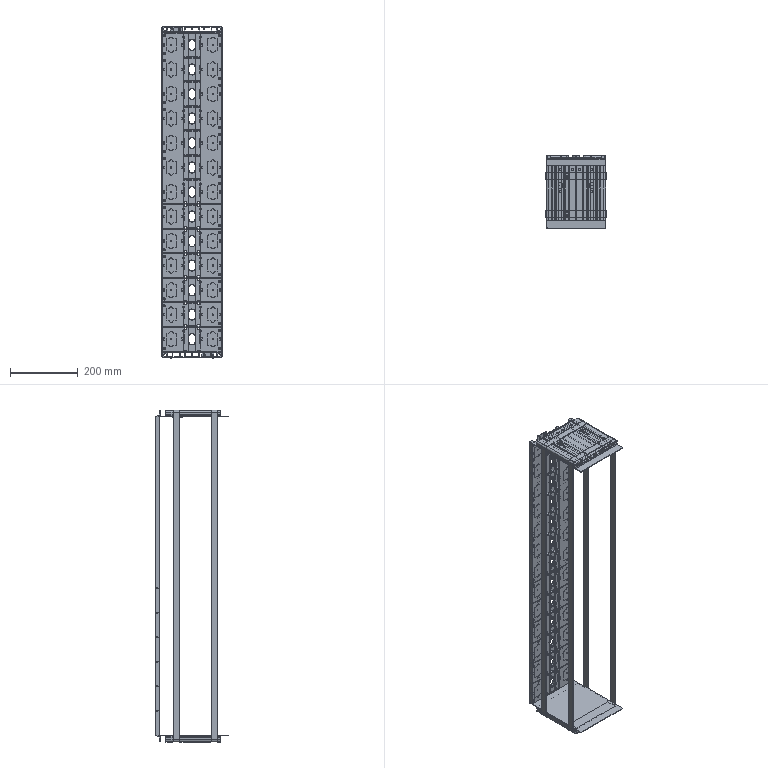Part | NX | features BREP 9 | 26 solids | 4992 faces | volume 1127254 mm3 | plane 2874 | cylinder 2118 | commonest cylinder face diameters 2 x433 4 x402 3 x208 0.6 x164 6 x130 10 x108